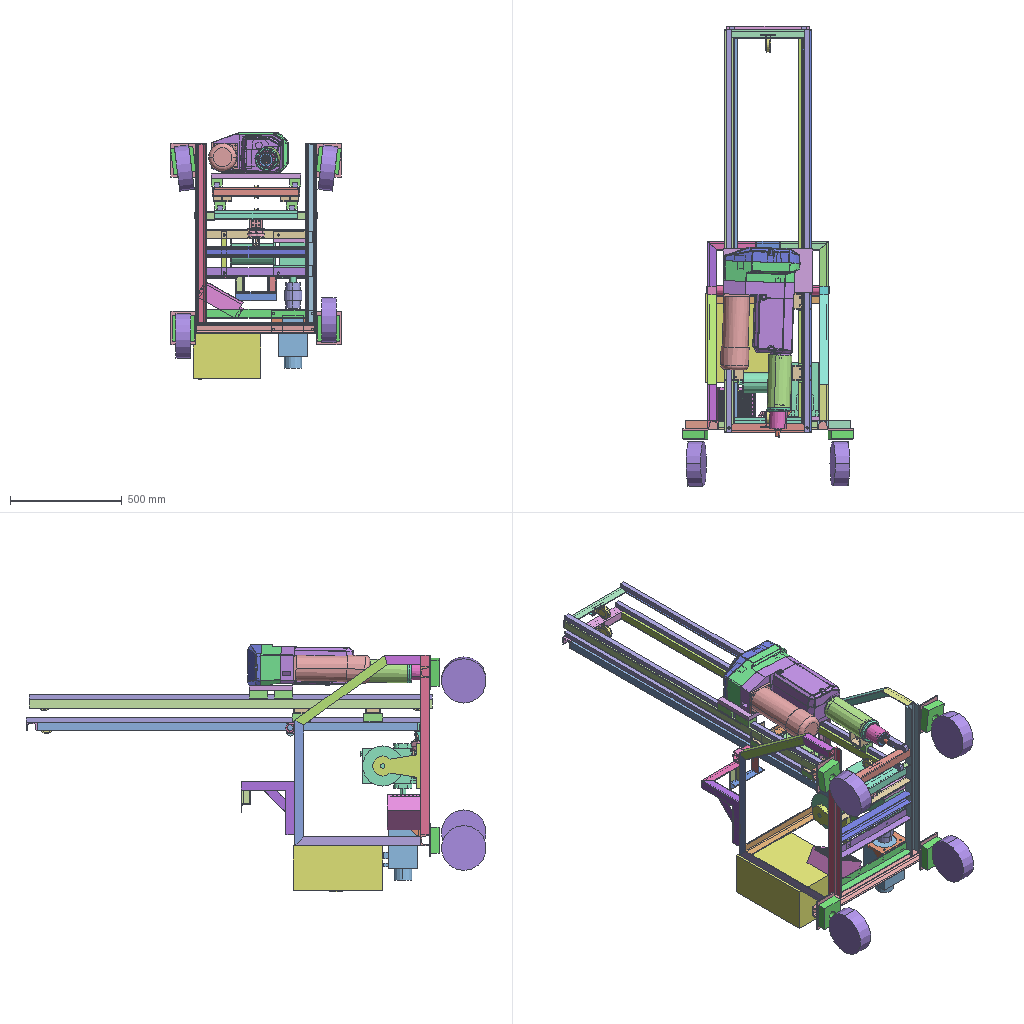Assembly | SolidWorks | 118 different items | 186 placed | box 763 x 2053 x 1107 mm
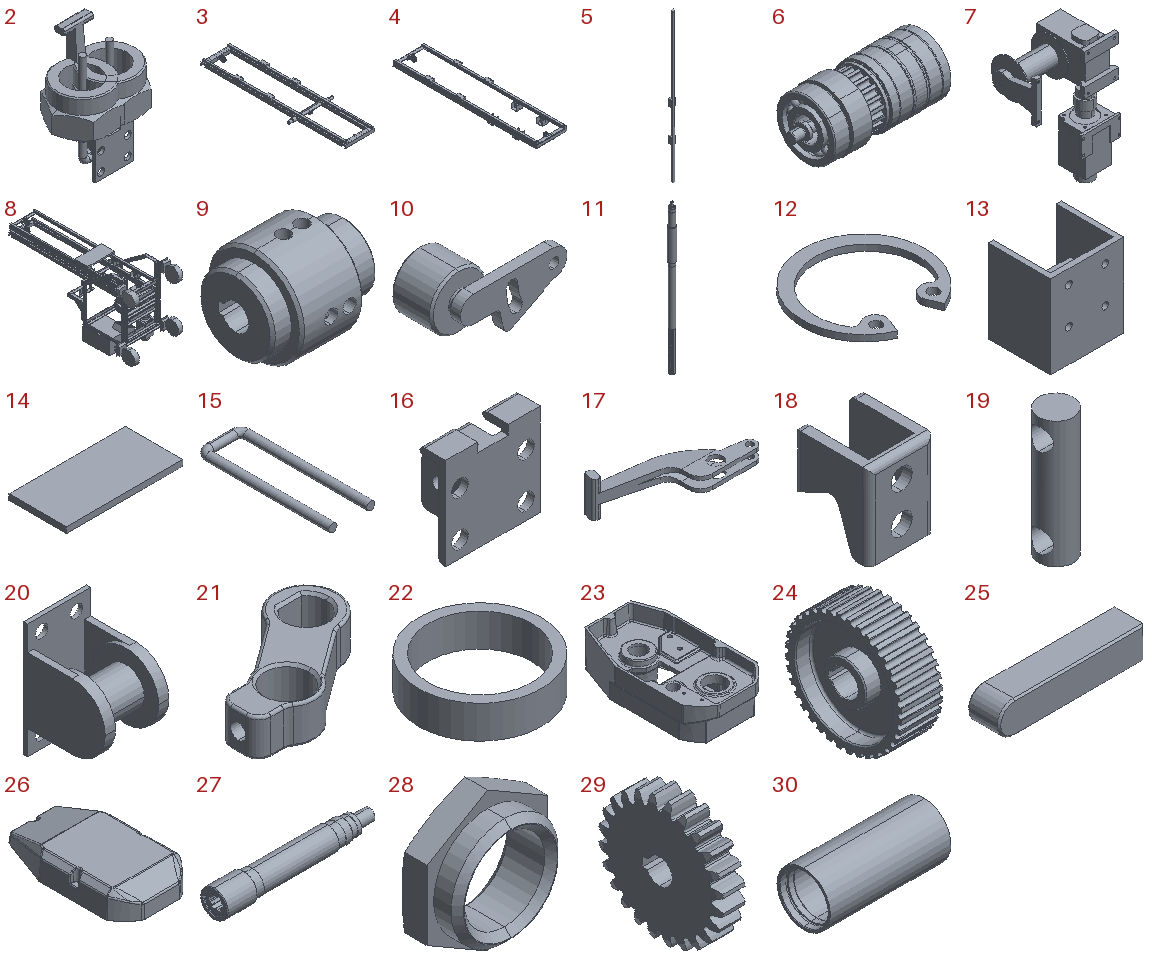Parts list (item | name | quantity | parent item | size | volume | features):
1 | (subassembly) | x1 | - | - | - | features CompositeCurve 39, AEMSimFeature 1
2 | (subassembly) | x1 | in 8 | 91.509 x 55.367 x 116.67 mm | 146833 mm3 | -
3 | (subassembly) | x1 | in 8 | 550 x 1800 x 100 mm | 5250915 mm3 | -
4 | (subassembly) | x1 | in 8 | 398 x 1800 x 104 mm | 4027094 mm3 | -
5 | (subassembly) | x4 | in 3, 4 | 48 x 40 x 1800 mm | 1122561 mm3 | -
6 | (subassembly) | x1 | in 1 | 155.5 x 64 x 64 mm | 413090 mm3 | features CompositeCurve 63
7 | (subassembly) | x1 | in 8 | 415 x 270 x 609 mm | 11625644 mm3 | -
8 | (subassembly) | x1 | - | 763.29 x 2055 x 1056 mm | 63128223 mm3 | -
9 | (subassembly) | x1 | in 1 | 41 x 36 x 36 mm | 28883 mm3 | features CompositeCurve 4
10 | (subassembly) | x1 | in 1 | 120.656 x 54 x 63.864 mm | 111745 mm3 | features CompositeCurve 20
11 | - | x1 | in 1 | 32 x 32 x 689 mm | 345284 mm3 | features ICE 14, Chamfer 8, CirPattern 1, Extrusion 1
12 | - | x2 | in 6 | 19.5 x 18.758 x 1 mm | 92.859 mm3 | features Extrusion 1
13 | - | x4 | in 4 | 70 x 60 x 80 mm | 83779 mm3 | features Cut 1, Extrusion 1, ICE 1
14 | - | x1 | in 8 | 398 x 195.319 x 20 mm | 1554736 mm3 | features Extrusion 1
15 | - | x1 | in 2 | 34 x 99 x 6 mm | 6099 mm3 | features Sweep 1
16 | - | x1 | in 2 | 40 x 27 x 39 mm | 8879 mm3 | features ICE 4, Extrusion 1, Fillet 1
17 | - | x1 | in 2 | 106.747 x 45.786 x 30 mm | 13050 mm3 | features Fillet 3, ICE 3, Extrusion 1
18 | - | x1 | in 3 | 20 x 23 x 26 mm | 3238 mm3 | features ICE 2, Extrusion 1, Fillet 1
19 | - | x1 | in 2 | 11 x 11 x 40 mm | 3000 mm3 | features Extrusion 1, ICE 1
20 | - | x1 | in 3 | 31 x 40 x 56 mm | 18443 mm3 | features ICE 3, MirrorPattern 1, Revolution 1
21 | - | x1 | in 1 | 121.493 x 89.432 x 30 mm | 103342 mm3 | features Fillet 2, Chamfer 1, Extrusion 1, ICE 1
22 | - | x1 | in 1 | 30 x 30 x 8 mm | 1728 mm3 | features Extrusion 1
23 | - | x1 | in 1 | 186.612 x 338.668 x 89.052 mm | 1423042 mm3 | features ICE 8, BaseBody 7, HoleWzd 2
24 | - | x1 | in 1 | 38.794 x 107.98 x 107.98 mm | 165804 mm3 | features Chamfer 3, ICE 2, CirPattern 1, Fillet 1, Revolution 1
25 | - | x2 | in 1 | 32 x 7 x 7 mm | 1519 mm3 | features Chamfer 1, Extrusion 1
26 | - | x1 | in 1 | 186.614 x 338.671 x 61.577 mm | 394276 mm3 | features BaseBody 7, ICE 7
27 | - | x1 | in 1 | 263 x 46 x 46 mm | 218227 mm3 | features BaseBody 3
28 | - | x2 | in 1 | 36 x 15 x 41.569 mm | 7224 mm3 | features Boss 1, RevCut 1, Revolution 1
29 | - | x1 | in 1 | 7.851 x 38.792 x 38.792 mm | 7390 mm3 | features Chamfer 2, ICE 2, CirPattern 1, Extrusion 1, RefAxis 1
30 | - | x1 | in 1 | 235 x 103.8 x 103.8 mm | 503241 mm3 | features Chamfer 2, Revolution 1
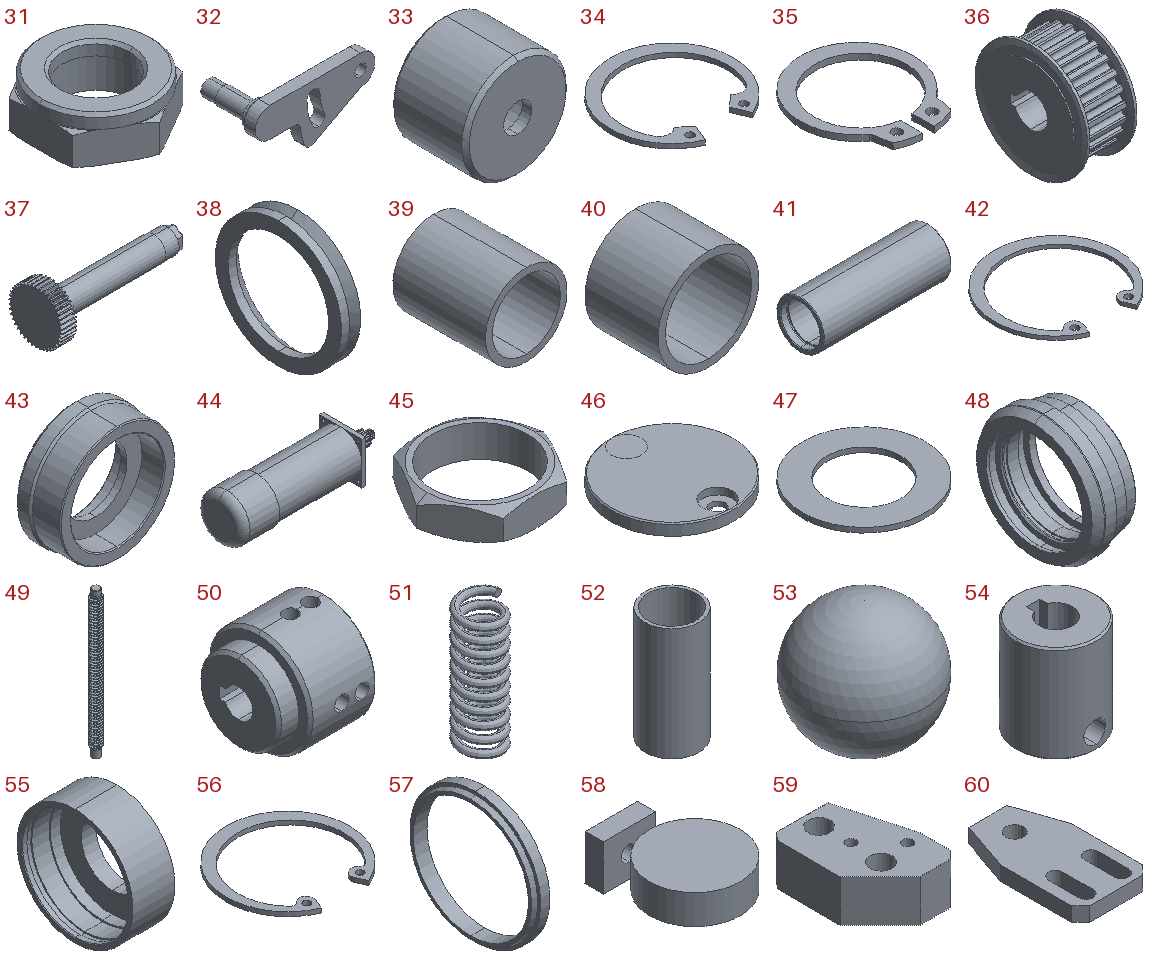31 | - | x2 | in 1 | 12.74 x 14.38 x 5 mm | 412.934 mm3 | features Cut 3, Boss 1, Chamfer 1, Extrusion 1
32 | - | x1 | in 10 | 105.906 x 54 x 49.114 mm | 37118 mm3 | features ICE 3, Fillet 2, Extrusion 1
33 | - | x1 | in 10 | 55.5 x 40 x 55.5 mm | 67056 mm3 | features Chamfer 1, Extrusion 1, ICE 1
34 | - | x1 | in 10 | 32.1 x 30.878 x 1.2 mm | 280.157 mm3 | features Extrusion 1
35 | - | x1 | in 10 | 19.4 x 21.927 x 1 mm | 117.841 mm3 | features Extrusion 1
36 | - | x1 | in 1 | 38 x 85.48 x 85.48 mm | 139347 mm3 | features ICE 2, CirPattern 1, Revolution 1
37 | - | x1 | in 1 | 144 x 54.909 x 55 mm | 94342 mm3 | features ICE 7, Chamfer 2, Fillet 2, CirPattern 1, Extrusion 1, RefAxis 1
38 | - | x1 | in 1 | 5.951 x 39 x 39 mm | 1479 mm3 | features Revolution 1
39 | - | x1 | in 1 | 30 x 34 x 30 mm | 7343 mm3 | features Extrusion 1
40 | - | x1 | in 1 | 47 x 34 x 47 mm | 16262 mm3 | features Extrusion 1
41 | - | x1 | in 1 | 202 x 75 x 75 mm | 280318 mm3 | features Chamfer 2, Revolution 1
42 | - | x1 | in 1 | 50.5 x 48.578 x 1.5 mm | 759.16 mm3 | features Extrusion 1
43 | - | x1 | in 1 | 64 x 24 x 64 mm | 33265 mm3 | features ICE 4, Chamfer 3, Extrusion 1, HoleWzd 1
44 | - | x1 | in 1 | 411 x 125 x 125 mm | 3738771 mm3 | features ICE 8, CirPattern 2, 3DProfileFeature 1, Extrusion 1, Fillet 1, HoleWzd 1, RefAxis 1
45 | - | x1 | in 1 | 48 x 41.569 x 12 mm | 5415 mm3 | features Extrusion 1, RevCut 1
46 | - | x1 | in 1 | 54 x 54 x 7.5 mm | 12264 mm3 | features 3DProfileFeature 1, Chamfer 1, Extrusion 1, HoleWzd 1, ICE 1
47 | - | x1 | in 1 | 30 x 30 x 1.2 mm | 542.867 mm3 | features Extrusion 1
48 | - | x1 | in 1 | 39 x 103.5 x 103.5 mm | 93923 mm3 | features Chamfer 3, Revolution 1
49 | - | x1 | in 1 | 14 x 14 x 189 mm | 21705 mm3 | features ICE 5, Chamfer 4, Extrusion 1, Helix 1, SweepCut 1
50 | - | x1 | in 9 | 30 x 36 x 36 mm | 17490 mm3 | features ICE 3, Chamfer 2, Revolution 1
51 | - | x1 | in 9 | 6 x 6 x 18 mm | 123.415 mm3 | features Helix 1, Sweep 1
52 | - | x1 | in 1 | 62 x 62 x 130 mm | 83621 mm3 | features Extrusion 1
53 | - | x2 | in 9 | 6 x 6 x 6 mm | 113.097 mm3 | features Revolution 1
54 | - | x1 | in 9 | 24 x 24 x 29 mm | 10899 mm3 | features ICE 3, Chamfer 2, Extrusion 1, HoleWzd 1
55 | - | x1 | in 1 | 21 x 47 x 47 mm | 7708 mm3 | features Chamfer 2, Revolution 1
56 | - | x1 | in 1 | 43.5 x 41.844 x 1.5 mm | 575.103 mm3 | features Extrusion 1
57 | - | x1 | in 1 | 9 x 85 x 85 mm | 9367 mm3 | features Revolution 1
58 | - | x4 | in 8 | 200 x 250 x 100 mm | 2463636 mm3 | features ICE 2, Extrusion 1
59 | - | x1 | in 1 | 39 x 55 x 21 mm | 33486 mm3 | features ICE 2, 3DProfileFeature 1, Extrusion 1, HoleWzd 1
60 | - | x1 | in 1 | 40 x 72 x 8 mm | 17211 mm3 | features Chamfer 1, Extrusion 1
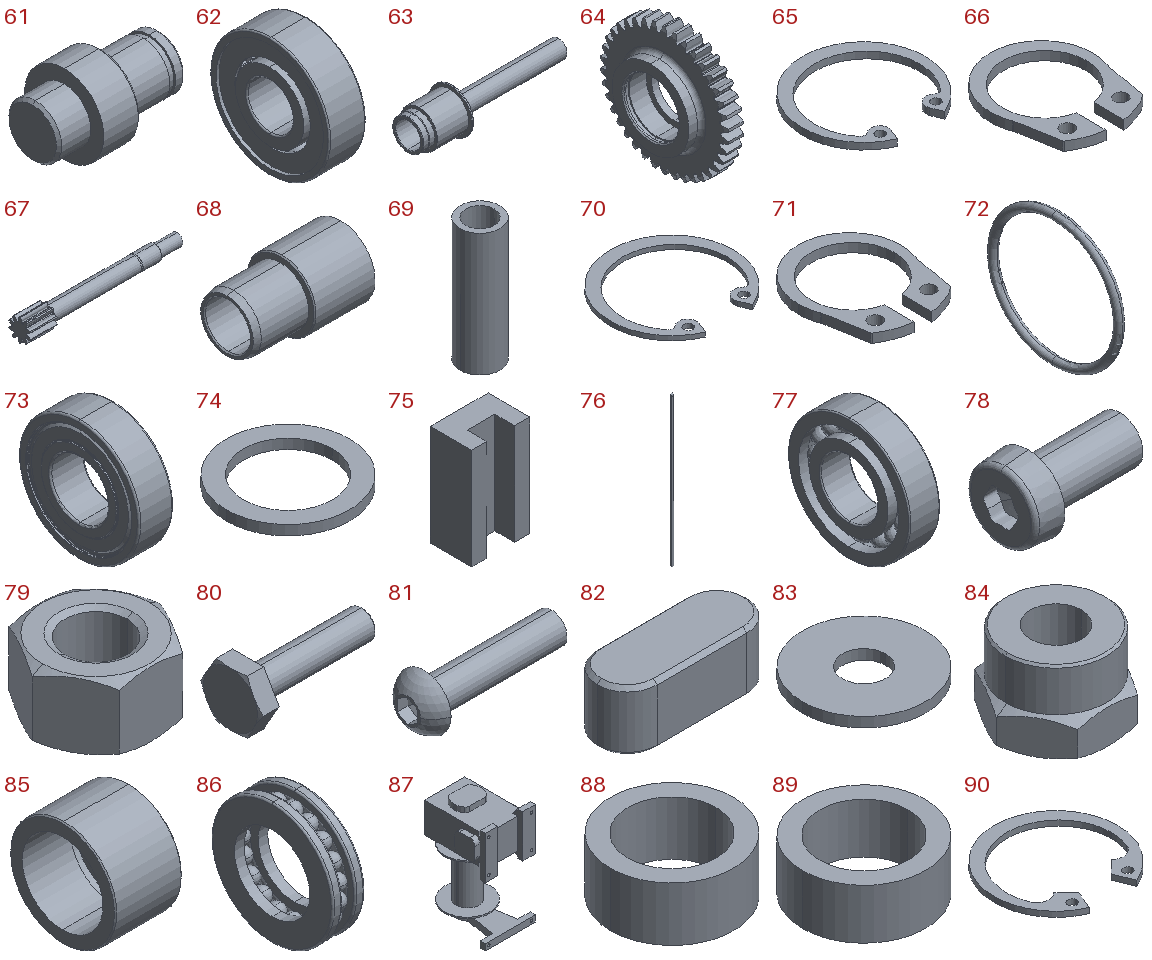61 | - | x1 | in 1 | 24 x 15 x 15 mm | 2547 mm3 | features ICE 4, Chamfer 3, Extrusion 1, RefAxis 1
62 | - | x1 | in 1 | 8 x 26 x 26 mm | 2223 mm3 | features Revolution 6, CirPattern 2, RevCut 2, Cut 1, MirrorSolid 1
63 | - | x1 | in 1 | 302.5 x 87 x 87 mm | 330300 mm3 | features BaseBody 2
64 | - | x1 | in 1 | 14 x 59.878 x 60 mm | 19418 mm3 | features Chamfer 3, ICE 2, CirPattern 1, Extrusion 1, Fillet 1, RefAxis 1, RevCut 1
65 | - | x1 | in 1 | 27.9 x 26.838 x 1.5 mm | 253.572 mm3 | features Extrusion 1
66 | - | x1 | in 1 | 11.5 x 13.997 x 1 mm | 53.264 mm3 | features Extrusion 1
67 | - | x1 | in 1 | 106 x 14.473 x 15 mm | 8561 mm3 | features ICE 7, Chamfer 2, CirPattern 1, Extrusion 1, RefAxis 1
68 | - | x1 | in 1 | 53 x 32 x 32 mm | 15205 mm3 | features Chamfer 1, Revolution 1
69 | - | x1 | in 1 | 14 x 14 x 43 mm | 3242 mm3 | features Extrusion 1
70 | - | x1 | in 1 | 27.9 x 26.838 x 1 mm | 169.048 mm3 | features Extrusion 1
71 | - | x1 | in 1 | 11.5 x 13.997 x 1 mm | 53.264 mm3 | features Extrusion 1
72 | - | x1 | in 1 | 5 x 85 x 85 mm | 4935 mm3 | features Revolution 1
73 | - | x1 | in 1 | 12 x 42 x 42 mm | 10321 mm3 | features BaseBody 1
74 | - | x1 | in 1 | 50 x 50 x 4 mm | 3782 mm3 | features Extrusion 1
75 | - | x8 | in 5 | 48 x 34.5 x 84 mm | 106558 mm3 | features Extrusion 1, HoleWzd 1
76 | - | x4 | in 5 | 23 x 22 x 1800 mm | 909444 mm3 | features ICE 2, Extrusion 1
77 | - | x20 | in 1, 6, 10 | 8 x 32 x 32 mm | 3760 mm3 | features Revolution 3, CirPattern 1, Fillet 1
78 | - | x4 | in 1 | 26 x 16 x 16 mm | 2561 mm3 | features BlendCut 1, Cut 1, Extrusion 1, Fillet 1, LPattern 1, RevCut 1, Revolution 1
79 | - | x3 | in 2, 10 | 24.249 x 21 x 12.8 mm | 3413 mm3 | features RevCut 2, Chamfer 1, Extrusion 1, LPattern 1
80 | - | x2 | in 1 | 11.825 x 5.566 x 4.82 mm | 84.307 mm3 | features RevCut 3, Boss 1, Chamfer 1, Extrusion 1, Fillet 1, LPattern 1
81 | - | x1 | in 1 | 56.6 x 21 x 21 mm | 6942 mm3 | features Cut 2, RevCut 2, Boss 1, Extrusion 1, Fillet 1, LPattern 1
82 | - | x7 | in 1, 6, 9 | 10 x 4 x 4 mm | 144.763 mm3 | features Boss 2, Chamfer 1, Extrusion 1
83 | - | x1 | in 1 | 37 x 37 x 3 mm | 2827 mm3 | features Extrusion 1
84 | - | x2 | in 2 | 11.547 x 10 x 8 mm | 473.326 mm3 | features RevCut 3, Boss 1, Chamfer 1, Extrusion 1, LPattern 1
85 | - | x1 | in 1 | 29 x 46 x 46 mm | 17975 mm3 | features Chamfer 1, Revolution 1
86 | - | x1 | in 1 | 11 x 42 x 42 mm | 7140 mm3 | features Revolution 3, CirPattern 1, Fillet 1
87 | - | x1 | in 7 | 250 x 270 x 405 mm | 7312574 mm3 | features ICE 11, Fillet 2, MirrorPattern 1, Revolution 1
88 | - | x1 | in 6 | 14 x 14 x 6.15 mm | 463.699 mm3 | features Extrusion 1
89 | - | x3 | in 6 | 14 x 14 x 5.7 mm | 429.77 mm3 | features Extrusion 1
90 | - | x1 | in 6 | 27.9 x 26.838 x 1.2 mm | 223.343 mm3 | features Extrusion 1
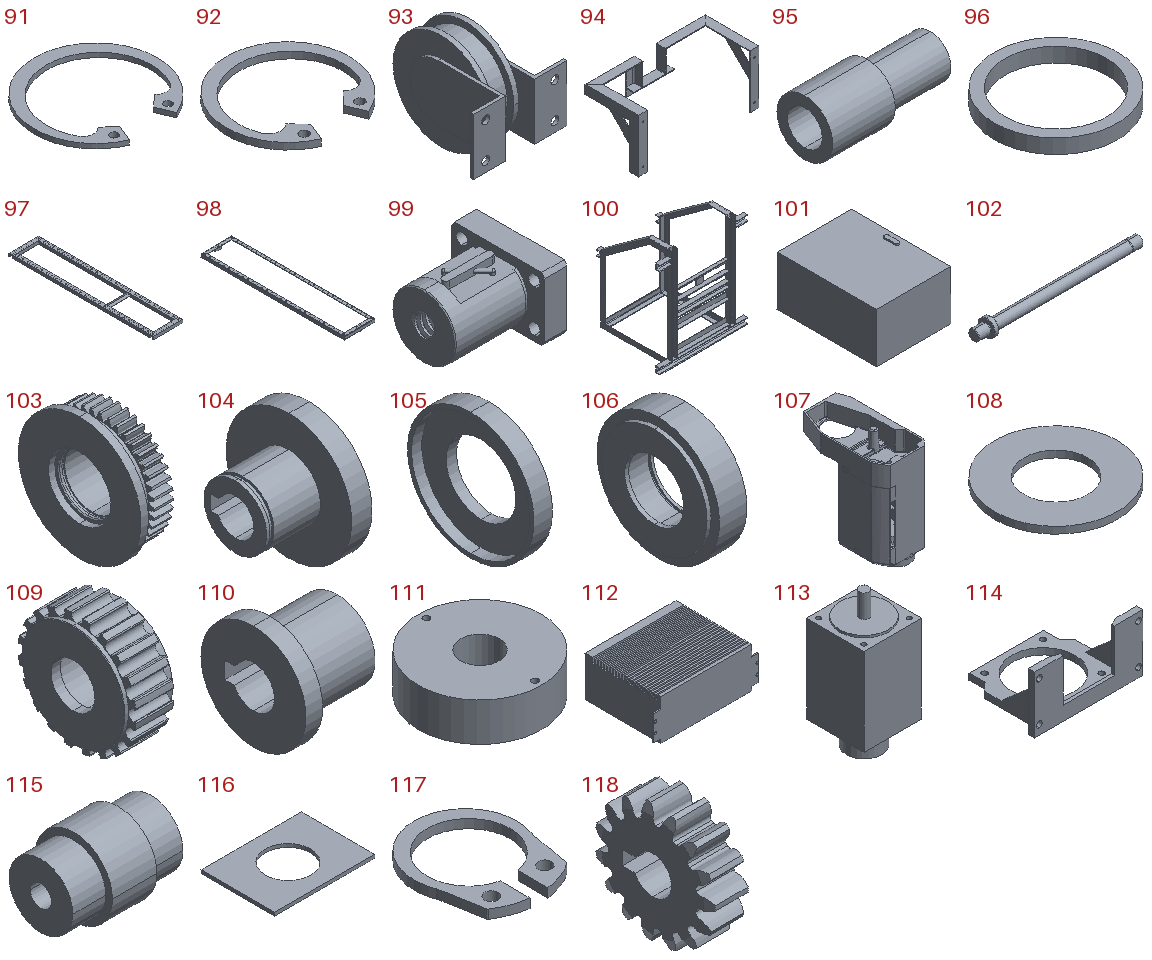91 | - | x2 | in 6 | 32.1 x 30.878 x 1.2 mm | 280.157 mm3 | features Extrusion 1
92 | - | x1 | in 6 | 27.9 x 26.838 x 1.5 mm | 279.179 mm3 | features Extrusion 1
93 | - | x3 | in 3, 4 | 58 x 70 x 60 mm | 52336 mm3 | features ICE 3, MirrorPattern 1, Revolution 1
94 | - | x1 | in 8 | 540 x 240 x 240 mm | 569268 mm3 | features ICE 2, 3DProfileFeature 1, MirrorPattern 1, WeldMemberFeat 1, WeldmentFeature 1
95 | - | x2 | in 3 | 90 x 40 x 40 mm | 44179 mm3 | features ICE 1, RefAxis 1, Revolution 1
96 | - | x1 | in 1 | 42.5 x 42.5 x 5 mm | 2283 mm3 | features Extrusion 1
97 | - | x1 | in 3 | 370 x 1800 x 37 mm | 2843417 mm3 | features ICE 3, WeldMemberFeat 1, WeldmentFeature 1
98 | - | x1 | in 4 | 390 x 1800 x 43 mm | 1342182 mm3 | features ICE 2, WeldMemberFeat 1, WeldmentFeature 1
99 | - | x1 | in 1 | 52 x 50 x 34 mm | 45697 mm3 | features ICE 8, Revolution 4, RefAxis 3, RevCut 2, 3DProfileFeature 1, Helix 1, SweepCut 1
100 | - | x1 | in 8 | 740 x 637 x 850 mm | 3794275 mm3 | features WeldMemberFeat 8, WeldCornerFeat 5, ICE 2, 3DProfileFeature 1, WeldmentFeature 1
101 | - | x1 | in 8 | 300 x 400 x 206 mm | 24005084 mm3 | features Extrusion 1, ICE 1
102 | - | x1 | in 6 | 155.5 x 16 x 16 mm | 12095 mm3 | features ICE 9, Chamfer 6, Extrusion 1, RefAxis 1
103 | - | x1 | in 6 | 24 x 58 x 58 mm | 29070 mm3 | features ICE 4, Chamfer 3, CirPattern 1, Extrusion 1, Fillet 1, RefAxis 1, RevCut 1
104 | - | x2 | in 6 | 20 x 34 x 34 mm | 6019 mm3 | features ICE 1, Revolution 1
105 | - | x2 | in 6 | 10 x 62 x 62 mm | 12064 mm3 | features Revolution 1
106 | - | x2 | in 6 | 14.9 x 58 x 58 mm | 27501 mm3 | features Revolution 1
107 | - | x1 | in 1 | 164.786 x 315.34 x 339.5 mm | 2454069 mm3 | features ICE 11, BaseBody 7, 3DProfileFeature 1, HoleWzd 1
108 | - | x1 | in 6 | 58 x 58 x 3.2 mm | 6193 mm3 | features Extrusion 1
109 | - | x1 | in 6 | 24 x 55.847 x 55.847 mm | 37187 mm3 | features Chamfer 1, CirPattern 1, ICE 1, Revolution 1
110 | - | x1 | in 6 | 20 x 25 x 25 mm | 4309 mm3 | features ICE 1, Revolution 1
111 | - | x1 | in 6 | 64 x 64 x 20 mm | 57715 mm3 | features Extrusion 1, HoleWzd 1
112 | - | x1 | in 8 | 208 x 150 x 80 mm | 2042108 mm3 | features ICE 6, Extrusion 1
113 | - | x1 | in 7 | 130 x 151 x 305 mm | 3625077 mm3 | features ICE 4, Extrusion 1
114 | - | x1 | in 7 | 190 x 145 x 100 mm | 268946 mm3 | features ICE 3, Extrusion 1, MirrorPattern 1
115 | - | x1 | in 7 | 114 x 80 x 80 mm | 419048 mm3 | features ICE 2, Revolution 1
116 | - | x4 | in 8 | 150 x 110 x 5 mm | 64431 mm3 | features Cut 1, Extrusion 1
117 | - | x1 | in 6 | 11.5 x 13.997 x 1 mm | 53.264 mm3 | features Extrusion 1
118 | - | x1 | in 1 | 8 x 25.314 x 25.444 mm | 2620 mm3 | features Chamfer 2, ICE 2, CirPattern 1, Extrusion 1, RefAxis 1
Mates (type | each side: item.copy, entity, surface, feature):
In the top assembly
Coincident | 14.1 face plane Boss-Extrude 1 | 23.1 face plane 输入7
In subassembly 8
Coincident | 3.1 plane | 8.1 plane
Coincident | 4.1 plane | 8.1 plane
Coincident | 75.1 face plane Boss-Extrude 1 | 13.1 face plane Boss-Extrude 1
Coincident | 116.1 face plane Boss-Extrude 1 | 58.1 face plane Boss-Extrude 2
Coincident | 100.1 face plane 结构Member 1 | 116.1 face plane Boss-Extrude 1
Coincident | 100.1 face plane 结构Member 3 | 116.1 face plane Boss-Extrude 1
Width | 116.1 face plane Boss-Extrude 1 | 116.1 face plane Boss-Extrude 1 | 100.1 face plane 结构Member 1 | 100.1 face plane 结构Member 1
Width | 58.1 face plane Boss-Extrude 2 | 58.1 face plane Boss-Extrude 2 | 116.1 face plane Boss-Extrude 1 | 116.1 face plane Boss-Extrude 1
Coincident | 100.1 face plane 结构Member 4 | 116.2 face plane Boss-Extrude 1
Coincident | 100.1 face plane 结构Member 3 | 116.2 face plane Boss-Extrude 1
Coincident | 100.1 face plane 结构Member 4 | 116.3 face plane Boss-Extrude 1
Coincident | 100.1 face plane 结构Member 2 | 116.3 face plane Boss-Extrude 1
Coincident | 100.1 face plane 结构Member 1 | 116.4 face plane Boss-Extrude 1
Coincident | 100.1 face plane 结构Member 2 | 116.4 face plane Boss-Extrude 1
Coincident | 116.1 face plane Boss-Extrude 1 | 116.4 face plane Boss-Extrude 1
Width | 116.2 face plane Boss-Extrude 1 | 116.2 face plane Boss-Extrude 1 | 100.1 face plane 结构Member 4 | 100.1 face plane 结构Member 4
Coincident | 116.2 face plane Boss-Extrude 1 | 116.3 face plane Boss-Extrude 1
Concentric | 116.2 face cylinder Cut-Extrude 1 | 58.2 face cylinder Cut-Extrude 1
Coincident | 116.2 face plane Boss-Extrude 1 | 58.2 face plane Boss-Extrude 2
Concentric | 116.3 face cylinder Cut-Extrude 1 | 58.3 face cylinder Cut-Extrude 1
Coincident | 116.3 face plane Boss-Extrude 1 | 58.3 face plane Boss-Extrude 2
Concentric | 116.4 face cylinder Cut-Extrude 1 | 58.4 face cylinder Cut-Extrude 1
Coincident | 116.4 face plane Boss-Extrude 1 | 58.4 face plane Boss-Extrude 2
Concentric | 58.1 face cylinder Cut-Extrude 1 | 116.1 face cylinder Cut-Extrude 1
Width | 75.1 face plane Boss-Extrude 1 | 75.1 face plane Boss-Extrude 1 | 13.1 face plane Boss-Extrude 1 | 13.1 face plane Boss-Extrude 1
Width | 13.2 face plane Boss-Extrude 1 | 13.2 face plane Boss-Extrude 1 | 75.2 face plane Boss-Extrude 1 | 75.2 face plane Boss-Extrude 1
Coincident | 100.1 face plane 结构Member 1 | 87.1 face plane Boss-Extrude 3
Coincident | 100.1 face plane 结构Member 6 | 113.1 face plane Boss-Extrude 1
DistanceDim | 113.1 face plane Boss-Extrude 5 | 100.1 face plane 结构Member 6
Coincident | 100.1 face plane 结构Member 6 | 94.1 face plane 结构Member 1 | 2 times
DistanceDim | 95.1 axis | 100.1 face plane 结构Member 7
DistanceDim | 95.1 axis | 100.1 face plane 结构Member 3
LimitDistanceDim | 13.2 face plane Boss-Extrude 1 | 97.1 face plane 结构Member 1
Coincident | 100.1 face plane 结构Member 2 | 112.1 face plane Boss-Extrude 1
Lock | 100.1 select_type:0 | 112.1 select_type:0
Coincident | 100.1 face plane Boss-Extrude 2 | 16.1 face plane Boss-Extrude 1
Coincident | 2.1 plane | 8.1 plane
Coincident | 100.1 face plane 结构Member 7 | 101.1 face plane Boss-Extrude 1
DistanceDim | 101.1 face plane Boss-Extrude 1 | 100.1 face plane 结构Member 5
DistanceDim | 100.1 face plane 结构Member 7 | 101.1 face plane Boss-Extrude 1
Parallel | 100.1 face plane 结构Member 6 | 97.1 face plane 结构Member 1
InPlace | 4.1 face plane Boss-Extrude 1 | 14.2 plane
In subassembly 7
Parallel | 113.2 face plane Boss-Extrude 1 | 87.2 face plane Boss-Extrude 3
Concentric | 113.2 face cylinder Boss-Extrude 3 | 87.2 face cylinder Boss-Extrude 6
Coincident | 113.2 face plane Boss-Extrude 1 | 114.1 face plane Boss-Extrude 1
Width | 114.1 face plane Boss-Extrude 1 | 114.1 face plane Boss-Extrude 1 | 113.2 face plane Boss-Extrude 1 | 113.2 face plane Boss-Extrude 1
Concentric | 113.2 face cylinder Boss-Extrude 2 | 114.1 face cylinder Boss-Extrude 1
Concentric | 87.2 face cylinder Boss-Extrude 6 | 115.1 face cylinder Cut-Extrude 2
DistanceDim | 114.1 face plane Boss-Extrude 1 | 115.1 face plane Revolve 1
DistanceDim | 115.1 face plane Revolve 1 | 87.2 face plane Boss-Extrude 5
In subassembly 2
Concentric | 16.2 face cylinder Cut-Extrude 2 | 17.1 face cylinder Boss-Extrude 1
Coincident | 17.1 plane | 2.2 plane
Concentric | 17.1 face cylinder Boss-Extrude 1 | 19.1 face cylinder Boss-Extrude 1
Coincident | 19.1 plane | 2.2 plane
Concentric | 19.1 face cylinder Cut-Extrude 1 | 15.1 face cylinder Sweep 1 | 2 times
Concentric | 15.1 face cylinder Sweep 1 | 84.1 face cylinder BaseNut
Concentric | 15.1 face cylinder Sweep 1 | 84.2 face cylinder BaseNut
Tangent | 19.1 face cylinder Boss-Extrude 1 | 84.1 face plane BaseNut
Concentric | 15.1 face cylinder Sweep 1 | 79.1 face cylinder BaseNut
Concentric | 15.1 face cylinder Sweep 1 | 79.2 face cylinder BaseNut
Coincident | 79.1 face plane BaseNut | 79.2 face plane BaseNut
Tangent | 19.1 face cylinder Boss-Extrude 1 | 79.2 face plane BaseNut
Coincident | 84.1 face plane Extrude1 | 84.2 face plane Extrude1
DistanceDim | 84.1 face plane Extrude1 | 15.1 face plane Sweep 1
In subassembly 3
Coincident | 97.2 face plane 结构Member 1 | 76.1 face plane Boss-Extrude 1 | 2 times
Width | 76.1 face plane Boss-Extrude 1 | 76.1 face plane Boss-Extrude 1 | 97.2 face plane 结构Member 1 | 97.2 face plane 结构Member 1
Coincident | 97.2 face plane 结构Member 1 | 76.2 face plane Boss-Extrude 1 | 2 times
Width | 76.2 face plane Boss-Extrude 1 | 76.2 face plane Boss-Extrude 1 | 97.2 face plane 结构Member 1 | 97.2 face plane 结构Member 1
Coincident | 75.3 face plane Boss-Extrude 1 | 75.4 face plane Boss-Extrude 1
Coincident | 75.5 face plane Boss-Extrude 1 | 75.6 face plane Boss-Extrude 1
Coincident | 97.2 face plane 结构Member 1 | 95.2 face plane Revolve 1
DistanceDim | 95.2 axis | 97.2 face plane 结构Member 1 | 2 times
Coincident | 97.2 face plane 结构Member 1 | 95.3 face plane Revolve 1
Coincident | 95.2 axis | 95.3 axis
Coincident | 97.2 face plane Boss-Extrude 1 | 20.1 face plane Boss-Extrude 1
Width | 20.1 face plane Boss-Extrude 1 | 20.1 face plane Mirror 1 | 97.2 face plane 结构Member 1 | 97.2 face plane 结构Member 1
Width | 20.1 face plane Boss-Extrude 2 | 20.1 face plane Boss-Extrude 2 | 97.2 face plane Boss-Extrude 1 | 97.2 face plane Boss-Extrude 1
Coincident | 97.2 face plane 结构Member 1 | 93.1 face plane Boss-Extrude 1
Width | 93.1 face plane Mirror 1 | 93.1 face plane Mirror 1 | 97.2 face plane 结构Member 1 | 97.2 face plane 结构Member 1
Width | 93.1 face plane Mirror 1 | 93.1 face plane Boss-Extrude 2 | 97.2 face plane 结构Member 1 | 97.2 face plane 结构Member 1
Coincident | 18.1 plane | 3.2 plane
Coincident | 97.2 face plane 结构Member 1 | 18.1 face plane Boss-Extrude 1
DistanceDim | 18.1 face plane Boss-Extrude 1 | 97.2 face plane 结构Member 1
In subassembly 5
Coincident | 75.7 face plane Boss-Extrude 1 | 75.8 face plane Boss-Extrude 1 | 2 times
Coincident | 75.7 plane | 5.1 plane
Coincident | 76.3 face plane Boss-Extrude 1 | 75.8 face plane Boss-Extrude 1
In subassembly 4
Coincident | 98.1 face plane 结构Member 1 | 76.1 face plane Boss-Extrude 1 | 2 times
Coincident | 98.1 face plane 结构Member 1 | 76.2 face plane Boss-Extrude 1 | 2 times
Width | 76.2 face plane Boss-Extrude 1 | 76.2 face plane Boss-Extrude 1 | 98.1 face plane 结构Member 1 | 98.1 face plane 结构Member 1
Width | 76.1 face plane Boss-Extrude 1 | 76.1 face plane Boss-Extrude 1 | 98.1 face plane 结构Member 1 | 98.1 face plane 结构Member 1
Coincident | 75.5 face plane Boss-Extrude 1 | 75.6 face plane Boss-Extrude 1
Coincident | 75.3 face plane Boss-Extrude 1 | 75.4 face plane Boss-Extrude 1
Coincident | 98.1 face plane 结构Member 1 | 13.3 face plane Boss-Extrude 1 | 2 times
Coincident | 98.1 face plane 结构Member 1 | 13.4 face plane Boss-Extrude 1 | 2 times
Coincident | 98.1 face plane 结构Member 1 | 13.5 face plane Boss-Extrude 1 | 2 times
Coincident | 98.1 face plane 结构Member 1 | 13.6 face plane Boss-Extrude 1 | 2 times
Coincident | 13.4 face plane Boss-Extrude 1 | 13.6 face plane Boss-Extrude 1
Coincident | 13.3 face plane Boss-Extrude 1 | 13.5 face plane Boss-Extrude 1
DistanceDim | 13.4 face plane Boss-Extrude 1 | 98.1 face plane 结构Member 1
DistanceDim | 13.3 face plane Boss-Extrude 1 | 13.4 face plane Boss-Extrude 1
Coincident | 98.1 face plane Boss-Extrude 1 | 93.1 face plane Mirror 1
Width | 93.1 face plane Boss-Extrude 2 | 93.1 face plane Mirror 1 | 98.1 face plane Boss-Extrude 1 | 98.1 face plane Boss-Extrude 1
Coincident | 98.1 face plane 结构Member 1 | 93.1 face plane Boss-Extrude 1
Coincident | 98.1 face plane Boss-Extrude 1 | 93.2 face plane Mirror 1
Coincident | 93.1 face plane Boss-Extrude 2 | 93.2 face plane Mirror 1
Coincident | 93.1 face plane Boss-Extrude 1 | 93.2 face plane Mirror 1
In subassembly 1
Concentric | 27.1 face cylinder 2工作轴Component-1-solid1 | 77.1 face cylinder Revolve2 | 2 times
Coincident | 27.1 face plane 2工作轴Component-1-solid1 | 77.1 face plane Revolve2
Coincident | 27.1 face cylinder 2工作轴Component-1-solid1 | 45.1 edge
Coincident | 45.1 face plane Boss-Extrude 1 | 77.1 face plane Revolve2
Concentric | 27.1 face cylinder 2工作轴Component-1-solid1 | 43.1 face cylinder Cut-Extrude 2
Coincident | 43.1 face plane Cut-Extrude 1 | 45.1 face plane Boss-Extrude 1
Concentric | 27.1 face cylinder 2工作轴Component-1-solid1 | 38.1 face cylinder Revolve 1
Coincident | 38.1 edge | 43.1 face plane Cut-Extrude 2
Concentric | 27.1 face cylinder 2工作轴Component-1-solid1 | 77.2 face cylinder Revolve2
Concentric | 27.1 face cylinder 2工作轴Component-1-solid1 | 52.1 face cylinder Boss-Extrude 1
Coincident | 52.1 face plane Boss-Extrude 1 | 77.2 face plane Revolve3
Coincident | 52.1 face plane Boss-Extrude 1 | 77.1 face plane Revolve3
Concentric | 30.1 face cylinder Revolve 2 | 52.1 face cylinder Boss-Extrude 1
Concentric | 41.1 face cylinder Revolve 1 | 52.1 face cylinder Boss-Extrude 1
Coincident | 41.1 face plane Revolve 1 | 43.1 face plane Boss-Extrude 1
Coincident | 27.1 face plane 2工作轴Component 23-1-solid1 | 11.1 face plane CirPattern 1
Coincident | 77.2 face plane Revolve3 | 63.1 face plane 14推进杆Component-1-solid1
Concentric | 41.1 face cylinder Revolve 1 | 48.1 face cylinder Revolve 1
Concentric | 48.1 face cylinder Revolve 1 | 72.1 select_type:24
Coincident | 48.1 face plane Revolve 1 | 72.1 select_type:24
Concentric | 41.1 face cylinder Revolve 1 | 57.1 face cylinder Revolve 1
Coincident | 48.1 face plane Revolve 1 | 57.1 face plane Revolve 1
Concentric | 30.1 face cylinder Revolve 2 | 41.1 face cylinder Revolve 1
Coincident | 30.1 face plane Revolve 2 | 48.1 face plane Revolve 1
Concentric | 63.1 face cylinder 14推进杆Component 2-1-solid1 | 1.1 select_type:0
Coincident | 63.1 face plane 14推进杆Component-1-solid1 | 1.1 face
Coincident | 48.1 face plane Revolve 1 | 1.1 face
Concentric | 30.1 face cylinder Revolve 2 | 96.1 face cylinder Boss-Extrude 1
Concentric | 63.1 face cylinder 14推进杆Component 2-1-solid1 | 85.1 face cylinder Revolve 1
Coincident | 85.1 face plane Revolve 1 | 96.1 face plane Boss-Extrude 1
Concentric | 63.1 face cylinder 14推进杆Component 2-1-solid1 | 74.1 face cylinder Boss-Extrude 1
Coincident | 63.1 face plane 14推进杆Component-1-solid1 | 74.1 face plane Boss-Extrude 1
Coincident | 74.1 face plane Boss-Extrude 1 | 85.1 edge
Concentric | 11.1 face cylinder Boss-Extrude 6 | 77.3 edge
Coincident | 11.1 face plane Boss-Extrude 6 | 77.3 face plane Revolve2
Concentric | 11.1 face cylinder Boss-Extrude 8 | 77.4 face cylinder Revolve2
Coincident | 11.1 face plane Boss-Extrude 6 | 77.4 face plane Revolve2
Concentric | 11.1 face cylinder Cut-Extrude 1 | 25.1 face cylinder Boss-Extrude 1
Coincident | 11.1 face plane Cut-Extrude 1 | 25.1 face plane Boss-Extrude 1 | 2 times
Concentric | 11.1 face cylinder Boss-Extrude 8 | 24.1 face cylinder Revolve 1
Coincident | 24.1 face plane Cut-Extrude 1 | 25.1 face plane Boss-Extrude 1
Concentric | 11.1 face cylinder Boss-Extrude 10 | 28.1 face cylinder Revolve 1
Concentric | 11.1 face cylinder Boss-Extrude 8 | 22.1 face cylinder Boss-Extrude 1
Coincident | 77.4 face plane Revolve2 | 22.1 face plane Boss-Extrude 1
Coincident | 24.1 face plane Revolve 1 | 22.1 face plane Boss-Extrude 1
Coincident | 24.1 face plane Revolve 1 | 28.1 face plane Revolve 1
Coincident | 11.1 face plane Cut-Extrude 2 | 82.1 face plane BaseKey | 2 times
Concentric | 11.1 face cylinder Cut-Extrude 2 | 82.1 face cylinder BaseKey
Concentric | 11.1 face cylinder Boss-Extrude 12 | 29.1 face cylinder Cut-Extrude 2
Coincident | 29.1 face plane Cut-Extrude 2 | 82.1 face plane BaseKey
Coincident | 11.1 face plane Boss-Extrude 11 | 29.1 face plane Boss-Extrude 1
Concentric | 11.1 face cylinder Boss-Extrude 12 | 31.1 face cylinder Base-Extrude
DistanceDim | 64.1 select_type:25 | 31.1 select_type:25
GearDim | 64.1 edge | 29.1 edge
Coincident | 29.1 face plane Boss-Extrude 1 | 64.1 face plane Boss-Extrude 1
Concentric | 60.1 face cylinder Boss-Extrude 1 | 61.1 face cylinder Boss-Extrude 2
Coincident | 60.1 face plane Boss-Extrude 1 | 61.1 face plane Boss-Extrude 2
Concentric | 61.1 face cylinder Boss-Extrude 3 | 62.1 face cylinder Boss-Revolve 4
Coincident | 61.1 face plane Boss-Extrude 2 | 62.1 face plane Boss-Revolve 4
Concentric | 61.1 face cylinder Boss-Extrude 5 | 66.1 face cylinder Base-Extrude
Coincident | 62.1 face plane Mirror所有1 | 66.1 face plane Base-Extrude
Concentric | 62.1 face cylinder Boss-Revolve 3 | 64.1 face cylinder Cut-Revolve 1
Coincident | 62.1 face plane Mirror所有1 | 64.1 face plane Cut-Revolve 1
Concentric | 61.1 face cylinder Boss-Extrude 2 | 65.1 edge
Coincident | 65.1 face plane Base-Extrude | 64.1 face plane Cut-Revolve 1
Coincident | 118.1 face plane Boss-Extrude 1 | 64.1 face plane Boss-Extrude 1
DistanceDim | 118.1 select_type:25 | 64.1 select_type:25
GearDim | 118.1 edge | 64.1 edge
Concentric | 118.1 face cylinder Cut-Extrude 2 | 67.1 face cylinder Boss-Extrude 3
Coincident | 67.1 face plane Cut-Extrude 2 | 82.2 face plane BaseKey | 2 times
Concentric | 67.1 face cylinder Cut-Extrude 2 | 82.2 face cylinder BaseKey
Coincident | 118.1 face plane Cut-Extrude 2 | 82.2 face plane BaseKey
Coincident | 118.1 face plane Boss-Extrude 1 | 67.1 face plane Boss-Extrude 5
Concentric | 67.1 face cylinder Boss-Extrude 6 | 31.2 face cylinder Base-Extrude
Coincident | 118.1 face plane Boss-Extrude 1 | 31.2 face plane Base-Extrude
Concentric | 67.1 face cylinder Boss-Extrude 3 | 77.5 face cylinder Revolve2
Concentric | 67.1 face cylinder Boss-Extrude 3 | 77.6 face cylinder Revolve2
Coincident | 67.1 face plane Boss-Extrude 1 | 77.5 face plane Revolve2
Concentric | 67.1 face cylinder Boss-Extrude 3 | 69.1 face cylinder Boss-Extrude 1
Coincident | 77.5 face plane Revolve2 | 69.1 face plane Boss-Extrude 1
Coincident | 69.1 face plane Boss-Extrude 1 | 77.6 face plane Revolve2
Concentric | 67.1 face cylinder Boss-Extrude 5 | 71.1 edge
Coincident | 71.1 face plane Base-Extrude | 77.6 face plane Revolve2
Concentric | 67.1 face cylinder Boss-Extrude 5 | 70.1 edge
Coincident | 70.1 face plane Base-Extrude | 77.6 face plane Revolve3
Concentric | 68.1 face cylinder Revolve 1 | 69.1 face cylinder Boss-Extrude 1
Coincident | 77.5 face plane Revolve3 | 68.1 face plane Revolve 1
Concentric | 1.1 face | 77.7 face cylinder Revolve2
Coincident | 1.1 face | 77.7 face plane Revolve2
Coincident | 67.1 face plane Boss-Extrude 1 | 1.1 face
Concentric | 77.7 face cylinder Revolve2 | 102.1 face cylinder Boss-Extrude 7 | 2 times
Coincident | 77.7 face plane Revolve2 | 117.1 face plane Base-Extrude
Coincident | 67.1 face plane Boss-Extrude 1 | 103.1 face plane Boss-Extrude 3
DistanceDim | 67.1 select_type:25 | 103.1 select_type:25
GearDim | 103.1 edge | 67.1 edge
Concentric | 102.1 face cylinder Boss-Extrude 1 | 54.1 face cylinder 大小mm 暗销Hole 2
Coincident | 77.8 face plane Revolve3 | 54.1 face plane Boss-Extrude 1
Concentric | 50.1 face cylinder Revolve 1 | 49.1 face cylinder Boss-Extrude 4
Coincident | 49.1 face plane Cut-Extrude 1 | 82.3 face plane BaseKey
Concentric | 49.1 face cylinder Cut-Extrude 1 | 82.3 face cylinder BaseKey
Parallel | 50.1 face plane Cut-Extrude 1 | 82.3 face plane BaseKey
Coincident | 50.1 face plane Revolve 1 | 49.1 face plane Extrude 1
Coincident | 49.1 edge | 77.9 face cylinder Revolve2
Concentric | 47.1 edge | 77.9 face cylinder Revolve3
Concentric | 46.1 edge | 77.9 face cylinder Revolve3
Coincident | 47.1 face plane Boss-Extrude 1 | 77.9 face plane Revolve3
Coincident | 46.1 face plane Boss-Extrude 1 | 47.1 face plane Boss-Extrude 1
Coincident | 49.1 face plane Extrude 1 | 77.9 face plane Revolve2
Concentric | 78.1 face cylinder Revolve1 | 59.1 face cylinder Cut-Extrude 1
Coincident | 78.1 face plane BaseHead | 59.1 face plane Cut-Extrude 1
Concentric | 59.1 face cylinder Cut-Extrude 2 | 78.2 face cylinder Revolve1
Coincident | 59.1 edge | 78.2 face plane BaseHead
Coincident | 60.1 face plane Boss-Extrude 1 | 59.1 face plane Boss-Extrude 1
Concentric | 59.1 face cylinder M6 Tapped Hole 1 | 80.1 face cylinder BaseBody
Coincident | 60.1 face plane Boss-Extrude 1 | 80.1 face plane BaseHead
Concentric | 59.1 edge | 80.2 face cylinder BaseBody
Coincident | 60.1 face plane Boss-Extrude 1 | 80.2 face plane BaseHead
Slot | 80.1 face cylinder BaseBody | 60.1 face cylinder Boss-Extrude 1
Slot | 80.2 face cylinder BaseBody | 60.1 face cylinder Boss-Extrude 1
Concentric | 54.1 face cylinder Boss-Extrude 1 | 55.1 face cylinder Revolve 1
Coincident | 77.8 face plane Revolve3 | 55.1 face plane Revolve 1
Concentric | 50.1 face cylinder Revolve 1 | 86.1 edge
Concentric | 50.1 face cylinder Revolve 1 | 56.1 edge
Coincident | 55.1 face plane Revolve 1 | 86.1 face plane Revolve2
Coincident | 55.1 face plane Revolve 1 | 56.1 face plane Base-Extrude
Concentric | 27.1 face cylinder 2工作轴Component-1-solid1 | 107.1 face cylinder Cut-Extrude 8
Coincident | 30.1 face plane Revolve 2 | 107.1 face plane Cut-Extrude 10
Coincident | 77.3 face plane Revolve3 | 107.1 face plane 输入7
Concentric | 111.1 face cylinder Boss-Extrude 1 | 107.1 face cylinder 输入7
Coincident | 107.1 face plane Cut-Extrude 6 | 23.2 face plane Cut-Extrude 6
Concentric | 77.7 face cylinder Revolve3 | 23.2 face cylinder 输入7
Concentric | 78.1 face cylinder Revolve1 | 23.2 face cylinder M6 Tapped Hole 1
Coincident | 107.1 face plane 输入7 | 44.1 face plane Boss-Extrude 5
Concentric | 107.1 face cylinder M6 Tapped Hole 1 | 44.1 face cylinder M8 Tapped Hole 1 | 2 times
Concentric | 1.1 face | 1.1 face
Coincident | 44.1 face plane Boss-Extrude 4 | 37.1 face plane Boss-Extrude 1
DistanceDim | 37.1 select_type:25 | 44.1 select_type:25
GearDim | 44.1 edge | 37.1 edge
Concentric | 39.1 face cylinder Boss-Extrude 1 | 37.1 face cylinder Boss-Extrude 4
Concentric | 40.1 face cylinder Boss-Extrude 1 | 37.1 face cylinder Boss-Extrude 4
Coincident | 39.1 face plane Boss-Extrude 1 | 40.1 face plane Boss-Extrude 1
Concentric | 1.1 edge | 37.1 face cylinder Boss-Extrude 4
Concentric | 37.1 face cylinder Boss-Extrude 4 | 77.10 face cylinder Revolve2
Coincident | 40.1 face plane Boss-Extrude 1 | 77.10 face plane Revolve3
Coincident | 1.1 face | 77.10 face plane Revolve3
Concentric | 37.1 face cylinder Boss-Extrude 4 | 42.1 edge
Coincident | 77.10 face plane Revolve3 | 42.1 face plane Base-Extrude
Concentric | 37.1 face cylinder Boss-Extrude 4 | 36.1 face cylinder Revolve 1
Concentric | 37.1 face cylinder Boss-Extrude 4 | 77.11 face cylinder Revolve2
Coincident | 40.1 face plane Boss-Extrude 1 | 77.11 face plane Revolve2
Coincident | 37.1 face plane Cut-Extrude 2 | 25.2 face plane Boss-Extrude 1
Concentric | 37.1 face cylinder Cut-Extrude 2 | 25.2 face cylinder Boss-Extrude 1
Parallel | 36.1 face plane Cut-Extrude 1 | 25.2 face plane Boss-Extrude 1
Coincident | 36.1 face plane Revolve 1 | 25.2 face plane Boss-Extrude 1
Concentric | 37.1 face cylinder Boss-Extrude 5 | 28.2 face cylinder Revolve 1
Coincident | 36.1 face plane Revolve 1 | 28.2 face plane Revolve 1
Coincident | 23.2 face plane 输入7 | 32.1 face plane Boss-Extrude 1
Concentric | 23.2 face cylinder M10x1.0 Tapped Hole 1 | 32.1 face cylinder Boss-Extrude 1
Concentric | 23.2 face cylinder M10x1.0 Tapped Hole 1 | 78.3 face cylinder Revolve1
Coincident | 32.1 face plane Boss-Extrude 1 | 78.3 face plane BaseHead
Concentric | 23.2 face cylinder M10x1.0 Tapped Hole 1 | 78.4 face cylinder Revolve1
Coincident | 32.1 face plane Boss-Extrude 1 | 78.4 face plane BaseHead
Coincident | 23.2 face plane Cut-Extrude 7 | 26.1 face plane Cut-Extrude 7
Concentric | 49.1 face cylinder Extrude 1 | 99.1 face cylinder Cut-Revolve 2
Screw | 49.1 face cylinder Extrude 1 | 99.1 face cylinder Cut-Revolve 2
Coincident | 63.1 face plane 14推进杆Component 2-1-solid1 | 99.1 face plane Revolve 1
Coincident | 99.1 face plane Boss-Extrude 1 | 21.1 face plane Boss-Extrude 1
Concentric | 99.1 face cylinder Revolve 1 | 21.1 face cylinder Boss-Extrude 1
Concentric | 63.1 face cylinder 14推进杆Component 2-1-solid1 | 21.1 face cylinder Boss-Extrude 1
Parallel | 99.1 face plane Cut-Extrude 5 | 21.1 edge
Coincident | 107.1 face plane 输入7 | 73.1 face plane BAY6004ZZ-SUS
Concentric | 21.1 face cylinder Cut-Extrude 1 | 73.1 face cylinder BAY6004ZZ-SUS
Concentric | 73.1 face cylinder BAY6004ZZ-SUS | 83.1 face cylinder Base-Extrude
Coincident | 73.1 face plane BAY6004ZZ-SUS | 83.1 edge
Concentric | 83.1 face cylinder Base-Extrude | 81.1 face cylinder BaseBody
Coincident | 83.1 face plane Base-Extrude | 81.1 face plane BaseHead
In subassembly 6
Concentric | 102.2 edge | 77.4 edge
Coincident | 102.2 face plane Boss-Extrude 3 | 77.4 face plane Revolve2
Concentric | 102.2 edge | 89.1 edge
Coincident | 77.4 face plane Revolve2 | 89.1 face plane Boss-Extrude 1
Concentric | 89.1 edge | 110.1 edge
Coincident | 89.1 face plane Boss-Extrude 1 | 110.1 face plane Revolve 1
Coincident | 102.2 face plane Cut-Extrude 3 | 82.4 face plane BaseKey
Coincident | 110.1 face plane Cut-Extrude 1 | 82.4 face plane BaseKey
Coincident | 102.2 face plane Cut-Extrude 2 | 82.1 face plane BaseKey
Concentric | 102.2 face cylinder Cut-Extrude 2 | 82.1 face cylinder BaseKey
Coincident | 102.2 face plane Cut-Extrude 2 | 82.2 face plane BaseKey
Concentric | 102.2 face cylinder Cut-Extrude 2 | 82.2 face cylinder BaseKey
Coincident | 77.12 face plane Revolve2 | 77.6 face plane Revolve2
Concentric | 77.12 edge | 77.6 edge
Coincident | 110.1 face plane Revolve 1 | 89.2 edge
Coincident | 110.1 edge | 89.2 edge
Coincident | 77.12 face plane Revolve2 | 89.2 face plane Boss-Extrude 1
Concentric | 110.1 edge | 111.2 edge
Coincident | 110.1 face plane Revolve 1 | 111.2 face plane Boss-Extrude 1
Concentric | 102.2 edge | 109.1 edge
Concentric | 109.1 edge | 92.1 edge
Coincident | 109.1 face plane Revolve 2 | 92.1 face plane Base-Extrude
Concentric | 77.6 edge | 89.3 edge
Coincident | 77.6 face plane Revolve2 | 89.3 face plane Boss-Extrude 1
Coincident | 109.1 edge | 108.1 edge
Concentric | 109.1 edge | 104.1 edge
Coincident | 108.1 face plane Boss-Extrude 1 | 104.1 face plane Revolve 1
Concentric | 77.5 edge | 104.1 edge
Concentric | 102.2 edge | 77.5 edge
Concentric | 102.2 edge | 77.10 edge
Concentric | 104.1 edge | 106.1 edge
Concentric | 104.1 edge | 91.1 edge
Coincident | 106.1 face plane Revolve 1 | 91.1 face plane Base-Extrude
Coincident | 77.5 face plane Revolve2 | 91.1 face plane Base-Extrude
Coincident | 77.5 face plane Revolve2 | 77.10 face plane Revolve2
Coincident | 104.1 face plane Revolve 1 | 106.1 face plane Revolve 1
Concentric | 105.1 edge | 106.1 edge
Coincident | 105.1 face plane Revolve 1 | 106.1 face plane Revolve 1
Concentric | 102.2 edge | 104.2 edge
Coincident | 104.1 face plane Revolve 1 | 104.2 face plane Revolve 1
Concentric | 104.2 edge | 12.1 edge
Coincident | 104.1 face plane Revolve 1 | 12.1 face plane Base-Extrude
Concentric | 12.2 edge | 104.2 edge
Coincident | 104.2 face plane Revolve 1 | 12.2 face plane Base-Extrude
Concentric | 102.2 edge | 77.7 edge
Concentric | 102.2 edge | 77.9 edge
Coincident | 77.7 face plane Revolve3 | 77.9 face plane Revolve3
Coincident | 77.7 face plane Revolve3 | 12.2 face plane Base-Extrude
Concentric | 102.2 edge | 106.2 edge
Concentric | 102.2 edge | 91.2 edge
Coincident | 106.2 face plane Revolve 1 | 91.2 face plane Base-Extrude
Coincident | 77.9 face plane Revolve3 | 91.2 face plane Base-Extrude
Concentric | 102.2 face cylinder Boss-Extrude 5 | 105.2 edge
Coincident | 105.2 face plane Revolve 1 | 106.2 face plane Revolve 1
Concentric | 102.2 edge | 103.2 edge
Concentric | 102.2 edge | 77.13 edge
Concentric | 102.2 edge | 77.11 edge
Coincident | 77.11 face plane Revolve3 | 77.13 face plane Revolve3
Coincident | 103.2 face plane Cut-Revolve 2 | 77.11 face plane Revolve3
Concentric | 102.2 edge | 88.1 edge
Coincident | 104.2 face plane Revolve 1 | 88.1 edge
Concentric | 102.2 edge | 90.1 edge
Coincident | 103.2 face plane Cut-Revolve 2 | 90.1 face plane Base-Extrude
Coincident | 88.1 face plane Boss-Extrude 1 | 77.13 face plane Revolve2
Concentric | 102.2 edge | 117.2 edge
Coincident | 102.2 face plane Boss-Extrude 5 | 117.2 face plane Base-Extrude
Concentric | 102.2 face cylinder Boss-Extrude 5 | 89.3 face cylinder Boss-Extrude 1
In subassembly 9
Concentric | 51.1 select_type:24 | 54.2 face cylinder Cut-Extrude 1
Concentric | 53.1 face sphere Revolve 1 | 54.2 face cylinder Cut-Extrude 1
Concentric | 54.2 face cylinder Cut-Extrude 1 | 53.2 face sphere Revolve 1
Concentric | 50.2 edge | 54.2 edge
Coincident | 50.2 face plane Revolve 1 | 54.2 face plane Boss-Extrude 1
Coincident | 82.5 face plane BaseKey | 54.2 face plane Cut-Extrude 3
Tangent | 54.2 face plane Boss-Extrude 1 | 82.5 face cylinder BaseKey
Coincident | 54.2 face plane Cut-Extrude 3 | 82.5 face plane BaseKey
In subassembly 10
Concentric | 32.2 edge | 77.14 edge
Concentric | 32.2 edge | 33.1 edge
Coincident | 32.2 face plane Boss-Extrude 2 | 33.1 face plane Boss-Extrude 1
Coincident | 33.1 face plane Boss-Extrude 2 | 77.14 face plane Revolve3
Concentric | 33.1 edge | 34.1 edge
Coincident | 34.1 face plane Base-Extrude | 77.14 face plane Revolve3
Concentric | 33.1 edge | 35.1 edge
Coincident | 77.14 face plane Revolve2 | 35.1 face plane Base-Extrude
Concentric | 33.1 edge | 79.2 edge
Coincident | 32.2 face plane Boss-Extrude 3 | 79.2 face plane BaseNut